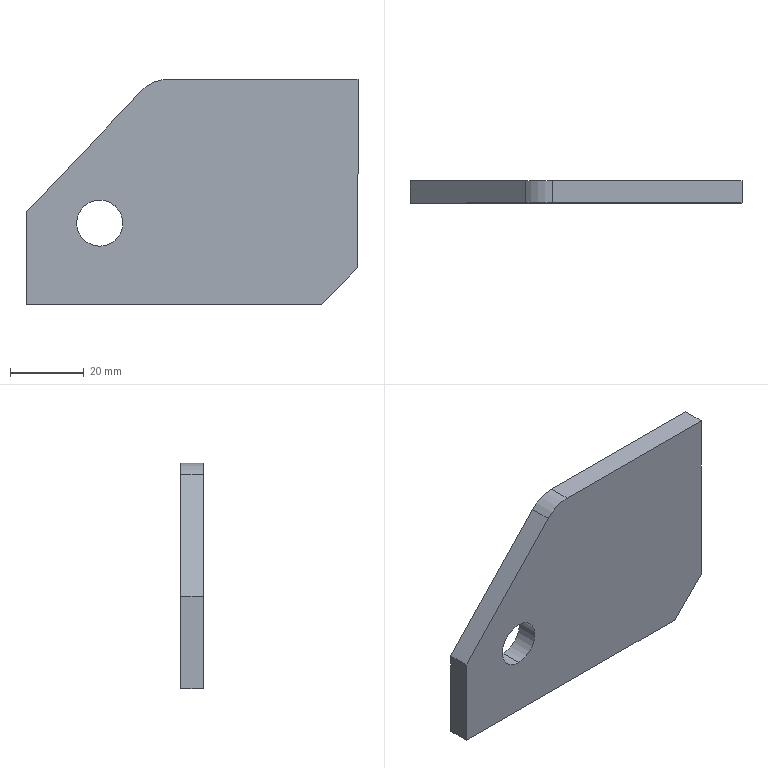Part | SolidWorks | features FlatPattern 1, SMBaseFlange 1, SheetMetal 1 | 1 solid | 11 faces | box 90 x 6 x 61.1 mm | volume 28229 mm3 | plane 8 | cylinder 3 | commonest cylinder face diameters 12.5 x2 20 x1
STEP:
#1=CARTESIAN_POINT('',(20.,6.,15.85));
#2=VERTEX_POINT('',#1);
#3=CARTESIAN_POINT('',(20.,6.,28.35));
#4=VERTEX_POINT('',#3);
#5=CARTESIAN_POINT('',(20.,6.,22.1));
#6=DIRECTION('',(0.,1.,0.));
#7=DIRECTION('',(0.,0.,1.));
#8=AXIS2_PLACEMENT_3D('',#5,#6,#7);
#9=CIRCLE('',#8,6.25);
#10=EDGE_CURVE('',#2,#4,#9,.T.);
#11=ORIENTED_EDGE('',*,*,#10,.T.);
#12=CARTESIAN_POINT('',(20.,0.,28.35));
#13=VERTEX_POINT('',#12);
#14=CARTESIAN_POINT('',(20.,6.,28.35));
#15=DIRECTION('',(0.,-1.,0.));
#16=VECTOR('',#15,1000.);
#17=LINE('',#14,#16);
#18=EDGE_CURVE('',#4,#13,#17,.T.);
#19=ORIENTED_EDGE('',*,*,#18,.T.);
#20=CARTESIAN_POINT('',(20.,0.,15.85));
#21=VERTEX_POINT('',#20);
#22=CARTESIAN_POINT('',(20.,0.,22.1));
#23=DIRECTION('',(0.,1.,0.));
#24=DIRECTION('',(0.,0.,1.));
#25=AXIS2_PLACEMENT_3D('',#22,#23,#24);
#26=CIRCLE('',#25,6.25);
#27=EDGE_CURVE('',#21,#13,#26,.T.);
#28=ORIENTED_EDGE('',*,*,#27,.F.);
#29=CARTESIAN_POINT('',(20.,6.,15.85));
#30=DIRECTION('',(0.,-1.,0.));
#31=VECTOR('',#30,1000.);
#32=LINE('',#29,#31);
#33=EDGE_CURVE('',#2,#21,#32,.T.);
#34=ORIENTED_EDGE('',*,*,#33,.F.);
#35=EDGE_LOOP('',(#11,#19,#28,#34));
#36=FACE_OUTER_BOUND('',#35,.T.);
#37=CARTESIAN_POINT('',(20.,6.,22.1));
#38=DIRECTION('',(0.,-1.,0.));
#39=DIRECTION('',(0.,0.,-1.));
#40=AXIS2_PLACEMENT_3D('',#37,#38,#39);
#41=CYLINDRICAL_SURFACE('',#40,6.25);
#42=ADVANCED_FACE('',(#36),#41,.F.);
#43=CARTESIAN_POINT('',(0.,6.,0.));
#44=VERTEX_POINT('',#43);
#45=CARTESIAN_POINT('',(0.,6.,25.));
#46=VERTEX_POINT('',#45);
#47=CARTESIAN_POINT('',(0.,6.,0.));
#48=DIRECTION('',(0.,0.,1.));
#49=VECTOR('',#48,1000.);
#50=LINE('',#47,#49);
#51=EDGE_CURVE('',#44,#46,#50,.T.);
#52=ORIENTED_EDGE('',*,*,#51,.T.);
#53=CARTESIAN_POINT('',(31.343,6.,57.988));
#54=VERTEX_POINT('',#53);
#55=CARTESIAN_POINT('',(0.,6.,25.));
#56=DIRECTION('',(0.6888,0.,0.7249));
#57=VECTOR('',#56,1000.);
#58=LINE('',#55,#57);
#59=EDGE_CURVE('',#46,#54,#58,.T.);
#60=ORIENTED_EDGE('',*,*,#59,.T.);
#61=CARTESIAN_POINT('',(38.593,6.,61.1));
#62=VERTEX_POINT('',#61);
#63=CARTESIAN_POINT('',(38.593,6.,51.1));
#64=DIRECTION('',(0.,1.,0.));
#65=DIRECTION('',(0.,0.,1.));
#66=AXIS2_PLACEMENT_3D('',#63,#64,#65);
#67=CIRCLE('',#66,10.);
#68=EDGE_CURVE('',#54,#62,#67,.T.);
#69=ORIENTED_EDGE('',*,*,#68,.T.);
#70=CARTESIAN_POINT('',(90.,6.,61.1));
#71=VERTEX_POINT('',#70);
#72=CARTESIAN_POINT('',(38.593,6.,61.1));
#73=DIRECTION('',(1.,0.,0.));
#74=VECTOR('',#73,1000.);
#75=LINE('',#72,#74);
#76=EDGE_CURVE('',#62,#71,#75,.T.);
#77=ORIENTED_EDGE('',*,*,#76,.T.);
#78=CARTESIAN_POINT('',(90.,6.,10.));
#79=VERTEX_POINT('',#78);
#80=CARTESIAN_POINT('',(90.,6.,10.));
#81=DIRECTION('',(0.,0.,-1.));
#82=VECTOR('',#81,1000.);
#83=LINE('',#80,#82);
#84=EDGE_CURVE('',#71,#79,#83,.T.);
#85=ORIENTED_EDGE('',*,*,#84,.T.);
#86=CARTESIAN_POINT('',(80.,6.,0.));
#87=VERTEX_POINT('',#86);
#88=CARTESIAN_POINT('',(80.,6.,0.));
#89=DIRECTION('',(-0.7071,0.,-0.7071));
#90=VECTOR('',#89,1000.);
#91=LINE('',#88,#90);
#92=EDGE_CURVE('',#79,#87,#91,.T.);
#93=ORIENTED_EDGE('',*,*,#92,.T.);
#94=CARTESIAN_POINT('',(0.,6.,0.));
#95=DIRECTION('',(-1.,0.,0.));
#96=VECTOR('',#95,1000.);
#97=LINE('',#94,#96);
#98=EDGE_CURVE('',#87,#44,#97,.T.);
#99=ORIENTED_EDGE('',*,*,#98,.T.);
#100=EDGE_LOOP('',(#52,#60,#69,#77,#85,#93,#99));
#101=FACE_OUTER_BOUND('',#100,.T.);
#102=ORIENTED_EDGE('',*,*,#10,.F.);
#103=CARTESIAN_POINT('',(20.,6.,22.1));
#104=DIRECTION('',(0.,1.,0.));
#105=DIRECTION('',(0.,0.,1.));
#106=AXIS2_PLACEMENT_3D('',#103,#104,#105);
#107=CIRCLE('',#106,6.25);
#108=EDGE_CURVE('',#4,#2,#107,.T.);
#109=ORIENTED_EDGE('',*,*,#108,.F.);
#110=EDGE_LOOP('',(#102,#109));
#111=FACE_BOUND('',#110,.T.);
#112=CARTESIAN_POINT('',(38.593,6.,51.1));
#113=DIRECTION('',(0.,1.,0.));
#114=DIRECTION('',(0.,0.,1.));
#115=AXIS2_PLACEMENT_3D('',#112,#113,#114);
#116=PLANE('',#115);
#117=ADVANCED_FACE('',(#101,#111),#116,.T.);
#118=CARTESIAN_POINT('',(0.,0.,0.));
#119=VERTEX_POINT('',#118);
#120=CARTESIAN_POINT('',(0.,0.,25.));
#121=VERTEX_POINT('',#120);
#122=CARTESIAN_POINT('',(0.,0.,0.));
#123=DIRECTION('',(0.,0.,1.));
#124=VECTOR('',#123,1000.);
#125=LINE('',#122,#124);
#126=EDGE_CURVE('',#119,#121,#125,.T.);
#127=ORIENTED_EDGE('',*,*,#126,.F.);
#128=CARTESIAN_POINT('',(80.,0.,0.));
#129=VERTEX_POINT('',#128);
#130=CARTESIAN_POINT('',(0.,0.,0.));
#131=DIRECTION('',(-1.,0.,0.));
#132=VECTOR('',#131,1000.);
#133=LINE('',#130,#132);
#134=EDGE_CURVE('',#129,#119,#133,.T.);
#135=ORIENTED_EDGE('',*,*,#134,.F.);
#136=CARTESIAN_POINT('',(90.,0.,10.));
#137=VERTEX_POINT('',#136);
#138=CARTESIAN_POINT('',(80.,0.,0.));
#139=DIRECTION('',(-0.7071,0.,-0.7071));
#140=VECTOR('',#139,1000.);
#141=LINE('',#138,#140);
#142=EDGE_CURVE('',#137,#129,#141,.T.);
#143=ORIENTED_EDGE('',*,*,#142,.F.);
#144=CARTESIAN_POINT('',(90.,0.,61.1));
#145=VERTEX_POINT('',#144);
#146=CARTESIAN_POINT('',(90.,0.,10.));
#147=DIRECTION('',(0.,0.,-1.));
#148=VECTOR('',#147,1000.);
#149=LINE('',#146,#148);
#150=EDGE_CURVE('',#145,#137,#149,.T.);
#151=ORIENTED_EDGE('',*,*,#150,.F.);
#152=CARTESIAN_POINT('',(38.593,0.,61.1));
#153=VERTEX_POINT('',#152);
#154=CARTESIAN_POINT('',(38.593,0.,61.1));
#155=DIRECTION('',(1.,0.,0.));
#156=VECTOR('',#155,1000.);
#157=LINE('',#154,#156);
#158=EDGE_CURVE('',#153,#145,#157,.T.);
#159=ORIENTED_EDGE('',*,*,#158,.F.);
#160=CARTESIAN_POINT('',(31.343,0.,57.988));
#161=VERTEX_POINT('',#160);
#162=CARTESIAN_POINT('',(38.593,0.,51.1));
#163=DIRECTION('',(0.,1.,0.));
#164=DIRECTION('',(0.,0.,1.));
#165=AXIS2_PLACEMENT_3D('',#162,#163,#164);
#166=CIRCLE('',#165,10.);
#167=EDGE_CURVE('',#161,#153,#166,.T.);
#168=ORIENTED_EDGE('',*,*,#167,.F.);
#169=CARTESIAN_POINT('',(0.,0.,25.));
#170=DIRECTION('',(0.6888,0.,0.7249));
#171=VECTOR('',#170,1000.);
#172=LINE('',#169,#171);
#173=EDGE_CURVE('',#121,#161,#172,.T.);
#174=ORIENTED_EDGE('',*,*,#173,.F.);
#175=EDGE_LOOP('',(#127,#135,#143,#151,#159,#168,#174));
#176=FACE_OUTER_BOUND('',#175,.T.);
#177=ORIENTED_EDGE('',*,*,#27,.T.);
#178=CARTESIAN_POINT('',(20.,0.,22.1));
#179=DIRECTION('',(0.,1.,0.));
#180=DIRECTION('',(0.,0.,1.));
#181=AXIS2_PLACEMENT_3D('',#178,#179,#180);
#182=CIRCLE('',#181,6.25);
#183=EDGE_CURVE('',#13,#21,#182,.T.);
#184=ORIENTED_EDGE('',*,*,#183,.T.);
#185=EDGE_LOOP('',(#177,#184));
#186=FACE_BOUND('',#185,.T.);
#187=CARTESIAN_POINT('',(38.593,0.,51.1));
#188=DIRECTION('',(0.,1.,0.));
#189=DIRECTION('',(0.,0.,1.));
#190=AXIS2_PLACEMENT_3D('',#187,#188,#189);
#191=PLANE('',#190);
#192=ADVANCED_FACE('',(#176,#186),#191,.F.);
#193=ORIENTED_EDGE('',*,*,#126,.T.);
#194=CARTESIAN_POINT('',(0.,6.,25.));
#195=DIRECTION('',(0.,-1.,0.));
#196=VECTOR('',#195,1000.);
#197=LINE('',#194,#196);
#198=EDGE_CURVE('',#46,#121,#197,.T.);
#199=ORIENTED_EDGE('',*,*,#198,.F.);
#200=ORIENTED_EDGE('',*,*,#51,.F.);
#201=CARTESIAN_POINT('',(0.,6.,0.));
#202=DIRECTION('',(0.,-1.,0.));
#203=VECTOR('',#202,1000.);
#204=LINE('',#201,#203);
#205=EDGE_CURVE('',#44,#119,#204,.T.);
#206=ORIENTED_EDGE('',*,*,#205,.T.);
#207=EDGE_LOOP('',(#193,#199,#200,#206));
#208=FACE_OUTER_BOUND('',#207,.T.);
#209=CARTESIAN_POINT('',(0.,6.,0.));
#210=DIRECTION('',(1.,0.,0.));
#211=DIRECTION('',(0.,0.,-1.));
#212=AXIS2_PLACEMENT_3D('',#209,#210,#211);
#213=PLANE('',#212);
#214=ADVANCED_FACE('',(#208),#213,.F.);
#215=ORIENTED_EDGE('',*,*,#173,.T.);
#216=CARTESIAN_POINT('',(31.343,6.,57.988));
#217=DIRECTION('',(0.,-1.,0.));
#218=VECTOR('',#217,1000.);
#219=LINE('',#216,#218);
#220=EDGE_CURVE('',#54,#161,#219,.T.);
#221=ORIENTED_EDGE('',*,*,#220,.F.);
#222=ORIENTED_EDGE('',*,*,#59,.F.);
#223=ORIENTED_EDGE('',*,*,#198,.T.);
#224=EDGE_LOOP('',(#215,#221,#222,#223));
#225=FACE_OUTER_BOUND('',#224,.T.);
#226=CARTESIAN_POINT('',(0.,6.,25.));
#227=DIRECTION('',(0.7249,0.,-0.6888));
#228=DIRECTION('',(-0.6888,0.,-0.7249));
#229=AXIS2_PLACEMENT_3D('',#226,#227,#228);
#230=PLANE('',#229);
#231=ADVANCED_FACE('',(#225),#230,.F.);
#232=ORIENTED_EDGE('',*,*,#167,.T.);
#233=CARTESIAN_POINT('',(38.593,6.,61.1));
#234=DIRECTION('',(0.,-1.,0.));
#235=VECTOR('',#234,1000.);
#236=LINE('',#233,#235);
#237=EDGE_CURVE('',#62,#153,#236,.T.);
#238=ORIENTED_EDGE('',*,*,#237,.F.);
#239=ORIENTED_EDGE('',*,*,#68,.F.);
#240=ORIENTED_EDGE('',*,*,#220,.T.);
#241=EDGE_LOOP('',(#232,#238,#239,#240));
#242=FACE_OUTER_BOUND('',#241,.T.);
#243=CARTESIAN_POINT('',(38.593,6.,51.1));
#244=DIRECTION('',(0.,-1.,0.));
#245=DIRECTION('',(0.,0.,-1.));
#246=AXIS2_PLACEMENT_3D('',#243,#244,#245);
#247=CYLINDRICAL_SURFACE('',#246,10.);
#248=ADVANCED_FACE('',(#242),#247,.T.);
#249=ORIENTED_EDGE('',*,*,#158,.T.);
#250=CARTESIAN_POINT('',(90.,6.,61.1));
#251=DIRECTION('',(0.,-1.,0.));
#252=VECTOR('',#251,1000.);
#253=LINE('',#250,#252);
#254=EDGE_CURVE('',#71,#145,#253,.T.);
#255=ORIENTED_EDGE('',*,*,#254,.F.);
#256=ORIENTED_EDGE('',*,*,#76,.F.);
#257=ORIENTED_EDGE('',*,*,#237,.T.);
#258=EDGE_LOOP('',(#249,#255,#256,#257));
#259=FACE_OUTER_BOUND('',#258,.T.);
#260=CARTESIAN_POINT('',(38.593,6.,61.1));
#261=DIRECTION('',(0.,0.,-1.));
#262=DIRECTION('',(-1.,0.,0.));
#263=AXIS2_PLACEMENT_3D('',#260,#261,#262);
#264=PLANE('',#263);
#265=ADVANCED_FACE('',(#259),#264,.F.);
#266=ORIENTED_EDGE('',*,*,#150,.T.);
#267=CARTESIAN_POINT('',(90.,6.,10.));
#268=DIRECTION('',(0.,-1.,0.));
#269=VECTOR('',#268,1000.);
#270=LINE('',#267,#269);
#271=EDGE_CURVE('',#79,#137,#270,.T.);
#272=ORIENTED_EDGE('',*,*,#271,.F.);
#273=ORIENTED_EDGE('',*,*,#84,.F.);
#274=ORIENTED_EDGE('',*,*,#254,.T.);
#275=EDGE_LOOP('',(#266,#272,#273,#274));
#276=FACE_OUTER_BOUND('',#275,.T.);
#277=CARTESIAN_POINT('',(90.,6.,10.));
#278=DIRECTION('',(-1.,0.,0.));
#279=DIRECTION('',(0.,0.,1.));
#280=AXIS2_PLACEMENT_3D('',#277,#278,#279);
#281=PLANE('',#280);
#282=ADVANCED_FACE('',(#276),#281,.F.);
#283=ORIENTED_EDGE('',*,*,#142,.T.);
#284=CARTESIAN_POINT('',(80.,6.,0.));
#285=DIRECTION('',(0.,-1.,0.));
#286=VECTOR('',#285,1000.);
#287=LINE('',#284,#286);
#288=EDGE_CURVE('',#87,#129,#287,.T.);
#289=ORIENTED_EDGE('',*,*,#288,.F.);
#290=ORIENTED_EDGE('',*,*,#92,.F.);
#291=ORIENTED_EDGE('',*,*,#271,.T.);
#292=EDGE_LOOP('',(#283,#289,#290,#291));
#293=FACE_OUTER_BOUND('',#292,.T.);
#294=CARTESIAN_POINT('',(80.,6.,0.));
#295=DIRECTION('',(-0.7071,0.,0.7071));
#296=DIRECTION('',(0.7071,0.,0.7071));
#297=AXIS2_PLACEMENT_3D('',#294,#295,#296);
#298=PLANE('',#297);
#299=ADVANCED_FACE('',(#293),#298,.F.);
#300=ORIENTED_EDGE('',*,*,#134,.T.);
#301=ORIENTED_EDGE('',*,*,#205,.F.);
#302=ORIENTED_EDGE('',*,*,#98,.F.);
#303=ORIENTED_EDGE('',*,*,#288,.T.);
#304=EDGE_LOOP('',(#300,#301,#302,#303));
#305=FACE_OUTER_BOUND('',#304,.T.);
#306=CARTESIAN_POINT('',(0.,6.,0.));
#307=DIRECTION('',(0.,0.,1.));
#308=DIRECTION('',(1.,0.,0.));
#309=AXIS2_PLACEMENT_3D('',#306,#307,#308);
#310=PLANE('',#309);
#311=ADVANCED_FACE('',(#305),#310,.F.);
#312=ORIENTED_EDGE('',*,*,#18,.F.);
#313=ORIENTED_EDGE('',*,*,#108,.T.);
#314=ORIENTED_EDGE('',*,*,#33,.T.);
#315=ORIENTED_EDGE('',*,*,#183,.F.);
#316=EDGE_LOOP('',(#312,#313,#314,#315));
#317=FACE_OUTER_BOUND('',#316,.T.);
#318=CARTESIAN_POINT('',(20.,6.,22.1));
#319=DIRECTION('',(0.,-1.,0.));
#320=DIRECTION('',(0.,0.,-1.));
#321=AXIS2_PLACEMENT_3D('',#318,#319,#320);
#322=CYLINDRICAL_SURFACE('',#321,6.25);
#323=ADVANCED_FACE('',(#317),#322,.F.);
#324=CLOSED_SHELL('',(#42,#117,#192,#214,#231,#248,#265,#282,#299,#311,#323));
#325=MANIFOLD_SOLID_BREP('',#324);
#326=CARTESIAN_POINT('',(0.,0.,0.));
#327=DIRECTION('',(0.,0.,1.));
#328=DIRECTION('',(1.,0.,0.));
#329=AXIS2_PLACEMENT_3D('',#326,#327,#328);
#330=(LENGTH_UNIT()NAMED_UNIT(*)SI_UNIT(.MILLI.,.METRE.));
#331=UNCERTAINTY_MEASURE_WITH_UNIT(LENGTH_MEASURE(0.00001),#330,'','');
#332=(NAMED_UNIT(*)PLANE_ANGLE_UNIT()SI_UNIT($,.RADIAN.));
#333=(NAMED_UNIT(*)SI_UNIT($,.STERADIAN.)SOLID_ANGLE_UNIT());
#334=(GEOMETRIC_REPRESENTATION_CONTEXT(3)GLOBAL_UNCERTAINTY_ASSIGNED_CONTEXT((#331))GLOBAL_UNIT_ASSIGNED_CONTEXT((#330,#332,#333))REPRESENTATION_CONTEXT('',''));
#335=ADVANCED_BREP_SHAPE_REPRESENTATION('',(#325,#329),#334);